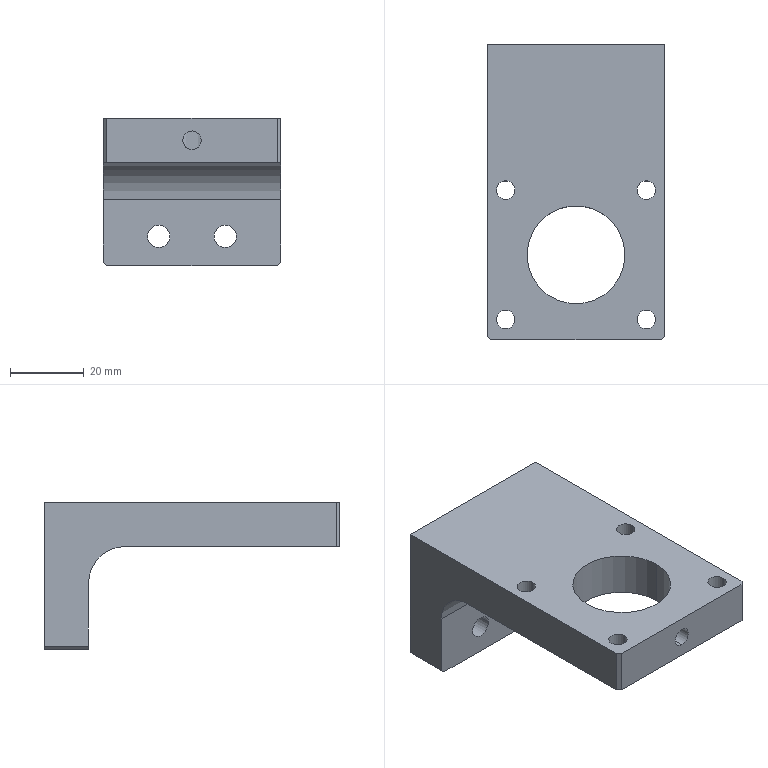Part | NX | features BREP 1 | 1 solid | 29 faces | box 48 x 80 x 40 mm | volume 54782 mm3 | cylinder 17 | plane 12 | commonest cylinder face diameters 5 x10 6 x4 26.5 x2 20 x1
STEP:
#1=CARTESIAN_POINT('',(0.,-30.25,2.5));
#2=VERTEX_POINT('',#1);
#3=CARTESIAN_POINT('',(0.,-30.25,-2.5));
#4=VERTEX_POINT('',#3);
#5=CARTESIAN_POINT('',(0.,-30.25,-2.5));
#6=CARTESIAN_POINT('',(-0.1554,-30.25,-2.5));
#7=CARTESIAN_POINT('',(-0.4644,-30.245,-2.477));
#8=CARTESIAN_POINT('',(-1.001,-30.214,-2.304));
#9=CARTESIAN_POINT('',(-1.293,-30.188,-2.154));
#10=CARTESIAN_POINT('',(-1.79,-30.132,-1.79));
#11=CARTESIAN_POINT('',(-2.16,-30.074,-1.284));
#12=CARTESIAN_POINT('',(-2.305,-30.048,-0.9992));
#13=CARTESIAN_POINT('',(-2.478,-30.017,-0.4608));
#14=CARTESIAN_POINT('',(-2.511,-30.01,0.001274));
#15=CARTESIAN_POINT('',(-2.478,-30.017,0.4638));
#16=CARTESIAN_POINT('',(-2.304,-30.048,1.002));
#17=CARTESIAN_POINT('',(-2.159,-30.074,1.286));
#18=CARTESIAN_POINT('',(-1.788,-30.132,1.793));
#19=CARTESIAN_POINT('',(-1.291,-30.188,2.155));
#20=CARTESIAN_POINT('',(-0.9972,-30.215,2.306));
#21=CARTESIAN_POINT('',(-0.4632,-30.245,2.477));
#22=CARTESIAN_POINT('',(-0.155,-30.25,2.5));
#23=CARTESIAN_POINT('',(0.,-30.25,2.5));
#24=B_SPLINE_CURVE_WITH_KNOTS('',3,(#5,#6,#7,#8,#9,#10,#11,#12,#13,#14,#15,#16,#17,#18,#19,#20,#21,#22,#23),.UNSPECIFIED.,.F.,.F.,(4,1,1,1,1,1,1,1,1,1,1,1,1,1,1,1,4),(0.,0.0625,0.125,0.1875,0.25,0.3125,0.375,0.4375,0.5,0.5625,0.625,0.6875,0.75,0.8125,0.875,0.9375,1.),.UNSPECIFIED.);
#25=EDGE_CURVE('',#2,#4,#24,.F.);
#26=ORIENTED_EDGE('',*,*,#25,.F.);
#27=CARTESIAN_POINT('',(0.,-40.,2.5));
#28=VERTEX_POINT('',#27);
#29=CARTESIAN_POINT('',(0.,-40.,2.5));
#30=DIRECTION('',(0.,-1.,0.));
#31=VECTOR('',#30,1000.);
#32=LINE('',#29,#31);
#33=EDGE_CURVE('',#2,#28,#32,.T.);
#34=ORIENTED_EDGE('',*,*,#33,.T.);
#35=CARTESIAN_POINT('',(0.,-40.,-2.5));
#36=VERTEX_POINT('',#35);
#37=CARTESIAN_POINT('',(0.,-40.,0.));
#38=DIRECTION('',(0.,-1.,0.));
#39=DIRECTION('',(0.,0.,-1.));
#40=AXIS2_PLACEMENT_3D('',#37,#38,#39);
#41=CIRCLE('',#40,2.5);
#42=EDGE_CURVE('',#28,#36,#41,.T.);
#43=ORIENTED_EDGE('',*,*,#42,.T.);
#44=CARTESIAN_POINT('',(0.,-40.,-2.5));
#45=DIRECTION('',(0.,-1.,0.));
#46=VECTOR('',#45,1000.);
#47=LINE('',#44,#46);
#48=EDGE_CURVE('',#4,#36,#47,.T.);
#49=ORIENTED_EDGE('',*,*,#48,.F.);
#50=EDGE_LOOP('',(#26,#34,#43,#49));
#51=FACE_BOUND('',#50,.T.);
#52=CARTESIAN_POINT('',(0.,-40.,0.));
#53=DIRECTION('',(0.,-1.,0.));
#54=DIRECTION('',(0.,0.,-1.));
#55=AXIS2_PLACEMENT_3D('',#52,#53,#54);
#56=CYLINDRICAL_SURFACE('',#55,2.5);
#57=ADVANCED_FACE('',(#51),#56,.F.);
#58=CARTESIAN_POINT('',(21.5,-34.5,6.));
#59=VERTEX_POINT('',#58);
#60=CARTESIAN_POINT('',(16.5,-34.5,6.));
#61=VERTEX_POINT('',#60);
#62=CARTESIAN_POINT('',(19.,-34.5,6.));
#63=DIRECTION('',(0.,0.,-1.));
#64=DIRECTION('',(1.,0.,0.));
#65=AXIS2_PLACEMENT_3D('',#62,#63,#64);
#66=CIRCLE('',#65,2.5);
#67=EDGE_CURVE('',#59,#61,#66,.T.);
#68=ORIENTED_EDGE('',*,*,#67,.F.);
#69=CARTESIAN_POINT('',(21.5,-34.5,-6.));
#70=VERTEX_POINT('',#69);
#71=CARTESIAN_POINT('',(21.5,-34.5,6.));
#72=DIRECTION('',(0.,0.,-1.));
#73=VECTOR('',#72,1000.);
#74=LINE('',#71,#73);
#75=EDGE_CURVE('',#59,#70,#74,.T.);
#76=ORIENTED_EDGE('',*,*,#75,.T.);
#77=CARTESIAN_POINT('',(16.5,-34.5,-6.));
#78=VERTEX_POINT('',#77);
#79=CARTESIAN_POINT('',(19.,-34.5,-6.));
#80=DIRECTION('',(0.,0.,-1.));
#81=DIRECTION('',(1.,0.,0.));
#82=AXIS2_PLACEMENT_3D('',#79,#80,#81);
#83=CIRCLE('',#82,2.5);
#84=EDGE_CURVE('',#70,#78,#83,.T.);
#85=ORIENTED_EDGE('',*,*,#84,.T.);
#86=CARTESIAN_POINT('',(16.5,-34.5,6.));
#87=DIRECTION('',(0.,0.,-1.));
#88=VECTOR('',#87,1000.);
#89=LINE('',#86,#88);
#90=EDGE_CURVE('',#61,#78,#89,.T.);
#91=ORIENTED_EDGE('',*,*,#90,.F.);
#92=EDGE_LOOP('',(#68,#76,#85,#91));
#93=FACE_BOUND('',#92,.T.);
#94=CARTESIAN_POINT('',(19.,-34.5,6.));
#95=DIRECTION('',(0.,0.,-1.));
#96=DIRECTION('',(-1.,0.,0.));
#97=AXIS2_PLACEMENT_3D('',#94,#95,#96);
#98=CYLINDRICAL_SURFACE('',#97,2.5);
#99=ADVANCED_FACE('',(#93),#98,.F.);
#100=CARTESIAN_POINT('',(21.5,0.5,6.));
#101=VERTEX_POINT('',#100);
#102=CARTESIAN_POINT('',(16.5,0.5,6.));
#103=VERTEX_POINT('',#102);
#104=CARTESIAN_POINT('',(19.,0.5,6.));
#105=DIRECTION('',(0.,0.,-1.));
#106=DIRECTION('',(1.,0.,0.));
#107=AXIS2_PLACEMENT_3D('',#104,#105,#106);
#108=CIRCLE('',#107,2.5);
#109=EDGE_CURVE('',#101,#103,#108,.T.);
#110=ORIENTED_EDGE('',*,*,#109,.F.);
#111=CARTESIAN_POINT('',(21.5,0.5,-6.));
#112=VERTEX_POINT('',#111);
#113=CARTESIAN_POINT('',(21.5,0.5,6.));
#114=DIRECTION('',(0.,0.,-1.));
#115=VECTOR('',#114,1000.);
#116=LINE('',#113,#115);
#117=EDGE_CURVE('',#101,#112,#116,.T.);
#118=ORIENTED_EDGE('',*,*,#117,.T.);
#119=CARTESIAN_POINT('',(16.5,0.5,-6.));
#120=VERTEX_POINT('',#119);
#121=CARTESIAN_POINT('',(19.,0.5,-6.));
#122=DIRECTION('',(0.,0.,-1.));
#123=DIRECTION('',(1.,0.,0.));
#124=AXIS2_PLACEMENT_3D('',#121,#122,#123);
#125=CIRCLE('',#124,2.5);
#126=EDGE_CURVE('',#112,#120,#125,.T.);
#127=ORIENTED_EDGE('',*,*,#126,.T.);
#128=CARTESIAN_POINT('',(16.5,0.5,6.));
#129=DIRECTION('',(0.,0.,-1.));
#130=VECTOR('',#129,1000.);
#131=LINE('',#128,#130);
#132=EDGE_CURVE('',#103,#120,#131,.T.);
#133=ORIENTED_EDGE('',*,*,#132,.F.);
#134=EDGE_LOOP('',(#110,#118,#127,#133));
#135=FACE_BOUND('',#134,.T.);
#136=CARTESIAN_POINT('',(19.,0.5,6.));
#137=DIRECTION('',(0.,0.,-1.));
#138=DIRECTION('',(-1.,0.,0.));
#139=AXIS2_PLACEMENT_3D('',#136,#137,#138);
#140=CYLINDRICAL_SURFACE('',#139,2.5);
#141=ADVANCED_FACE('',(#135),#140,.F.);
#142=CARTESIAN_POINT('',(-16.5,0.5,6.));
#143=VERTEX_POINT('',#142);
#144=CARTESIAN_POINT('',(-21.5,0.5,6.));
#145=VERTEX_POINT('',#144);
#146=CARTESIAN_POINT('',(-19.,0.5,6.));
#147=DIRECTION('',(0.,0.,-1.));
#148=DIRECTION('',(-1.,0.,0.));
#149=AXIS2_PLACEMENT_3D('',#146,#147,#148);
#150=CIRCLE('',#149,2.5);
#151=EDGE_CURVE('',#143,#145,#150,.T.);
#152=ORIENTED_EDGE('',*,*,#151,.F.);
#153=CARTESIAN_POINT('',(-16.5,0.5,-6.));
#154=VERTEX_POINT('',#153);
#155=CARTESIAN_POINT('',(-16.5,0.5,6.));
#156=DIRECTION('',(0.,0.,-1.));
#157=VECTOR('',#156,1000.);
#158=LINE('',#155,#157);
#159=EDGE_CURVE('',#143,#154,#158,.T.);
#160=ORIENTED_EDGE('',*,*,#159,.T.);
#161=CARTESIAN_POINT('',(-21.5,0.5,-6.));
#162=VERTEX_POINT('',#161);
#163=CARTESIAN_POINT('',(-19.,0.5,-6.));
#164=DIRECTION('',(0.,0.,-1.));
#165=DIRECTION('',(-1.,0.,0.));
#166=AXIS2_PLACEMENT_3D('',#163,#164,#165);
#167=CIRCLE('',#166,2.5);
#168=EDGE_CURVE('',#154,#162,#167,.T.);
#169=ORIENTED_EDGE('',*,*,#168,.T.);
#170=CARTESIAN_POINT('',(-21.5,0.5,6.));
#171=DIRECTION('',(0.,0.,-1.));
#172=VECTOR('',#171,1000.);
#173=LINE('',#170,#172);
#174=EDGE_CURVE('',#145,#162,#173,.T.);
#175=ORIENTED_EDGE('',*,*,#174,.F.);
#176=EDGE_LOOP('',(#152,#160,#169,#175));
#177=FACE_BOUND('',#176,.T.);
#178=CARTESIAN_POINT('',(-19.,0.5,6.));
#179=DIRECTION('',(0.,0.,-1.));
#180=DIRECTION('',(-1.,0.,0.));
#181=AXIS2_PLACEMENT_3D('',#178,#179,#180);
#182=CYLINDRICAL_SURFACE('',#181,2.5);
#183=ADVANCED_FACE('',(#177),#182,.F.);
#184=CARTESIAN_POINT('',(-16.5,-34.5,6.));
#185=VERTEX_POINT('',#184);
#186=CARTESIAN_POINT('',(-21.5,-34.5,6.));
#187=VERTEX_POINT('',#186);
#188=CARTESIAN_POINT('',(-19.,-34.5,6.));
#189=DIRECTION('',(0.,0.,-1.));
#190=DIRECTION('',(-1.,0.,0.));
#191=AXIS2_PLACEMENT_3D('',#188,#189,#190);
#192=CIRCLE('',#191,2.5);
#193=EDGE_CURVE('',#185,#187,#192,.T.);
#194=ORIENTED_EDGE('',*,*,#193,.F.);
#195=CARTESIAN_POINT('',(-16.5,-34.5,-6.));
#196=VERTEX_POINT('',#195);
#197=CARTESIAN_POINT('',(-16.5,-34.5,6.));
#198=DIRECTION('',(0.,0.,-1.));
#199=VECTOR('',#198,1000.);
#200=LINE('',#197,#199);
#201=EDGE_CURVE('',#185,#196,#200,.T.);
#202=ORIENTED_EDGE('',*,*,#201,.T.);
#203=CARTESIAN_POINT('',(-21.5,-34.5,-6.));
#204=VERTEX_POINT('',#203);
#205=CARTESIAN_POINT('',(-19.,-34.5,-6.));
#206=DIRECTION('',(0.,0.,-1.));
#207=DIRECTION('',(-1.,0.,0.));
#208=AXIS2_PLACEMENT_3D('',#205,#206,#207);
#209=CIRCLE('',#208,2.5);
#210=EDGE_CURVE('',#196,#204,#209,.T.);
#211=ORIENTED_EDGE('',*,*,#210,.T.);
#212=CARTESIAN_POINT('',(-21.5,-34.5,6.));
#213=DIRECTION('',(0.,0.,-1.));
#214=VECTOR('',#213,1000.);
#215=LINE('',#212,#214);
#216=EDGE_CURVE('',#187,#204,#215,.T.);
#217=ORIENTED_EDGE('',*,*,#216,.F.);
#218=EDGE_LOOP('',(#194,#202,#211,#217));
#219=FACE_BOUND('',#218,.T.);
#220=CARTESIAN_POINT('',(-19.,-34.5,6.));
#221=DIRECTION('',(0.,0.,-1.));
#222=DIRECTION('',(-1.,0.,0.));
#223=AXIS2_PLACEMENT_3D('',#220,#221,#222);
#224=CYLINDRICAL_SURFACE('',#223,2.5);
#225=ADVANCED_FACE('',(#219),#224,.F.);
#226=CARTESIAN_POINT('',(6.,40.,-26.));
#227=VERTEX_POINT('',#226);
#228=CARTESIAN_POINT('',(12.,40.,-26.));
#229=VERTEX_POINT('',#228);
#230=CARTESIAN_POINT('',(9.,40.,-26.));
#231=DIRECTION('',(0.,-1.,0.));
#232=DIRECTION('',(0.,0.,-1.));
#233=AXIS2_PLACEMENT_3D('',#230,#231,#232);
#234=CIRCLE('',#233,3.);
#235=EDGE_CURVE('',#227,#229,#234,.T.);
#236=ORIENTED_EDGE('',*,*,#235,.F.);
#237=CARTESIAN_POINT('',(6.,28.,-26.));
#238=VERTEX_POINT('',#237);
#239=CARTESIAN_POINT('',(6.,58.,-26.));
#240=DIRECTION('',(0.,-1.,0.));
#241=VECTOR('',#240,1000.);
#242=LINE('',#239,#241);
#243=EDGE_CURVE('',#238,#227,#242,.F.);
#244=ORIENTED_EDGE('',*,*,#243,.F.);
#245=CARTESIAN_POINT('',(12.,28.,-26.));
#246=VERTEX_POINT('',#245);
#247=CARTESIAN_POINT('',(9.,28.,-26.));
#248=DIRECTION('',(0.,-1.,0.));
#249=DIRECTION('',(1.,0.,0.));
#250=AXIS2_PLACEMENT_3D('',#247,#248,#249);
#251=CIRCLE('',#250,3.);
#252=EDGE_CURVE('',#238,#246,#251,.T.);
#253=ORIENTED_EDGE('',*,*,#252,.T.);
#254=CARTESIAN_POINT('',(12.,58.,-26.));
#255=DIRECTION('',(0.,-1.,0.));
#256=VECTOR('',#255,1000.);
#257=LINE('',#254,#256);
#258=EDGE_CURVE('',#246,#229,#257,.F.);
#259=ORIENTED_EDGE('',*,*,#258,.T.);
#260=EDGE_LOOP('',(#236,#244,#253,#259));
#261=FACE_BOUND('',#260,.T.);
#262=CARTESIAN_POINT('',(9.,58.,-26.));
#263=DIRECTION('',(0.,-1.,0.));
#264=DIRECTION('',(1.,0.,0.));
#265=AXIS2_PLACEMENT_3D('',#262,#263,#264);
#266=CYLINDRICAL_SURFACE('',#265,3.);
#267=ADVANCED_FACE('',(#261),#266,.F.);
#268=CARTESIAN_POINT('',(-12.,40.,-26.));
#269=VERTEX_POINT('',#268);
#270=CARTESIAN_POINT('',(-6.,40.,-26.));
#271=VERTEX_POINT('',#270);
#272=CARTESIAN_POINT('',(-9.,40.,-26.));
#273=DIRECTION('',(0.,-1.,0.));
#274=DIRECTION('',(0.,0.,-1.));
#275=AXIS2_PLACEMENT_3D('',#272,#273,#274);
#276=CIRCLE('',#275,3.);
#277=EDGE_CURVE('',#269,#271,#276,.T.);
#278=ORIENTED_EDGE('',*,*,#277,.F.);
#279=CARTESIAN_POINT('',(-12.,28.,-26.));
#280=VERTEX_POINT('',#279);
#281=CARTESIAN_POINT('',(-12.,58.,-26.));
#282=DIRECTION('',(0.,-1.,0.));
#283=VECTOR('',#282,1000.);
#284=LINE('',#281,#283);
#285=EDGE_CURVE('',#280,#269,#284,.F.);
#286=ORIENTED_EDGE('',*,*,#285,.F.);
#287=CARTESIAN_POINT('',(-6.,28.,-26.));
#288=VERTEX_POINT('',#287);
#289=CARTESIAN_POINT('',(-9.,28.,-26.));
#290=DIRECTION('',(0.,-1.,0.));
#291=DIRECTION('',(1.,0.,0.));
#292=AXIS2_PLACEMENT_3D('',#289,#290,#291);
#293=CIRCLE('',#292,3.);
#294=EDGE_CURVE('',#280,#288,#293,.T.);
#295=ORIENTED_EDGE('',*,*,#294,.T.);
#296=CARTESIAN_POINT('',(-6.,58.,-26.));
#297=DIRECTION('',(0.,-1.,0.));
#298=VECTOR('',#297,1000.);
#299=LINE('',#296,#298);
#300=EDGE_CURVE('',#288,#271,#299,.F.);
#301=ORIENTED_EDGE('',*,*,#300,.T.);
#302=EDGE_LOOP('',(#278,#286,#295,#301));
#303=FACE_BOUND('',#302,.T.);
#304=CARTESIAN_POINT('',(-9.,58.,-26.));
#305=DIRECTION('',(0.,-1.,0.));
#306=DIRECTION('',(1.,0.,0.));
#307=AXIS2_PLACEMENT_3D('',#304,#305,#306);
#308=CYLINDRICAL_SURFACE('',#307,3.);
#309=ADVANCED_FACE('',(#303),#308,.F.);
#310=CARTESIAN_POINT('',(-13.25,-17.,-6.));
#311=VERTEX_POINT('',#310);
#312=CARTESIAN_POINT('',(13.25,-17.,-6.));
#313=VERTEX_POINT('',#312);
#314=CARTESIAN_POINT('',(0.,-17.,-6.));
#315=DIRECTION('',(0.,0.,1.));
#316=DIRECTION('',(1.,0.,0.));
#317=AXIS2_PLACEMENT_3D('',#314,#315,#316);
#318=CIRCLE('',#317,13.25);
#319=EDGE_CURVE('',#311,#313,#318,.T.);
#320=ORIENTED_EDGE('',*,*,#319,.F.);
#321=CARTESIAN_POINT('',(-13.25,-17.,6.));
#322=VERTEX_POINT('',#321);
#323=CARTESIAN_POINT('',(-13.25,-17.,-6.));
#324=DIRECTION('',(0.,0.,1.));
#325=VECTOR('',#324,1000.);
#326=LINE('',#323,#325);
#327=EDGE_CURVE('',#322,#311,#326,.F.);
#328=ORIENTED_EDGE('',*,*,#327,.F.);
#329=CARTESIAN_POINT('',(13.25,-17.,6.));
#330=VERTEX_POINT('',#329);
#331=CARTESIAN_POINT('',(0.,-17.,6.));
#332=DIRECTION('',(0.,0.,1.));
#333=DIRECTION('',(1.,0.,0.));
#334=AXIS2_PLACEMENT_3D('',#331,#332,#333);
#335=CIRCLE('',#334,13.25);
#336=EDGE_CURVE('',#322,#330,#335,.T.);
#337=ORIENTED_EDGE('',*,*,#336,.T.);
#338=CARTESIAN_POINT('',(13.25,-17.,-6.));
#339=DIRECTION('',(0.,0.,1.));
#340=VECTOR('',#339,1000.);
#341=LINE('',#338,#340);
#342=EDGE_CURVE('',#330,#313,#341,.F.);
#343=ORIENTED_EDGE('',*,*,#342,.T.);
#344=EDGE_LOOP('',(#320,#328,#337,#343));
#345=FACE_BOUND('',#344,.T.);
#346=CARTESIAN_POINT('',(0.,-30.25,-2.5));
#347=CARTESIAN_POINT('',(0.6639,-30.25,-2.5));
#348=CARTESIAN_POINT('',(1.954,-30.132,-1.958));
#349=CARTESIAN_POINT('',(2.773,-29.952,-0.001957));
#350=CARTESIAN_POINT('',(1.954,-30.132,1.96));
#351=CARTESIAN_POINT('',(0.6633,-30.25,2.5));
#352=CARTESIAN_POINT('',(0.,-30.25,2.5));
#353=B_SPLINE_CURVE_WITH_KNOTS('',3,(#346,#347,#348,#349,#350,#351,#352),.UNSPECIFIED.,.F.,.F.,(4,1,1,1,4),(0.,0.25,0.5,0.75,1.),.UNSPECIFIED.);
#354=EDGE_CURVE('',#4,#2,#353,.T.);
#355=ORIENTED_EDGE('',*,*,#354,.T.);
#356=ORIENTED_EDGE('',*,*,#25,.T.);
#357=EDGE_LOOP('',(#355,#356));
#358=FACE_BOUND('',#357,.T.);
#359=CARTESIAN_POINT('',(0.,-17.,-6.));
#360=DIRECTION('',(0.,0.,1.));
#361=DIRECTION('',(1.,0.,0.));
#362=AXIS2_PLACEMENT_3D('',#359,#360,#361);
#363=CYLINDRICAL_SURFACE('',#362,13.25);
#364=ADVANCED_FACE('',(#345,#358),#363,.F.);
#365=CARTESIAN_POINT('',(-24.,18.,-6.));
#366=VERTEX_POINT('',#365);
#367=CARTESIAN_POINT('',(-24.,-39.,-6.));
#368=VERTEX_POINT('',#367);
#369=CARTESIAN_POINT('',(-24.,-40.,-6.));
#370=DIRECTION('',(0.,-1.,0.));
#371=VECTOR('',#370,1000.);
#372=LINE('',#369,#371);
#373=EDGE_CURVE('',#366,#368,#372,.T.);
#374=ORIENTED_EDGE('',*,*,#373,.F.);
#375=CARTESIAN_POINT('',(24.,18.,-6.));
#376=VERTEX_POINT('',#375);
#377=CARTESIAN_POINT('',(24.,18.,-6.));
#378=DIRECTION('',(1.,0.,0.));
#379=VECTOR('',#378,1000.);
#380=LINE('',#377,#379);
#381=EDGE_CURVE('',#366,#376,#380,.T.);
#382=ORIENTED_EDGE('',*,*,#381,.T.);
#383=CARTESIAN_POINT('',(24.,-39.,-6.));
#384=VERTEX_POINT('',#383);
#385=CARTESIAN_POINT('',(24.,-40.,-6.));
#386=DIRECTION('',(0.,1.,0.));
#387=VECTOR('',#386,1000.);
#388=LINE('',#385,#387);
#389=EDGE_CURVE('',#384,#376,#388,.T.);
#390=ORIENTED_EDGE('',*,*,#389,.F.);
#391=CARTESIAN_POINT('',(23.,-40.,-6.));
#392=VERTEX_POINT('',#391);
#393=CARTESIAN_POINT('',(24.,-39.,-6.));
#394=DIRECTION('',(-0.7071,-0.7071,0.));
#395=VECTOR('',#394,1000.);
#396=LINE('',#393,#395);
#397=EDGE_CURVE('',#384,#392,#396,.T.);
#398=ORIENTED_EDGE('',*,*,#397,.T.);
#399=CARTESIAN_POINT('',(-23.,-40.,-6.));
#400=VERTEX_POINT('',#399);
#401=CARTESIAN_POINT('',(24.,-40.,-6.));
#402=DIRECTION('',(1.,0.,0.));
#403=VECTOR('',#402,1000.);
#404=LINE('',#401,#403);
#405=EDGE_CURVE('',#400,#392,#404,.T.);
#406=ORIENTED_EDGE('',*,*,#405,.F.);
#407=CARTESIAN_POINT('',(-23.,-40.,-6.));
#408=DIRECTION('',(-0.7071,0.7071,0.));
#409=VECTOR('',#408,1000.);
#410=LINE('',#407,#409);
#411=EDGE_CURVE('',#400,#368,#410,.T.);
#412=ORIENTED_EDGE('',*,*,#411,.T.);
#413=EDGE_LOOP('',(#374,#382,#390,#398,#406,#412));
#414=FACE_BOUND('',#413,.T.);
#415=CARTESIAN_POINT('',(19.,-34.5,-6.));
#416=DIRECTION('',(0.,0.,-1.));
#417=DIRECTION('',(1.,0.,0.));
#418=AXIS2_PLACEMENT_3D('',#415,#416,#417);
#419=CIRCLE('',#418,2.5);
#420=EDGE_CURVE('',#78,#70,#419,.T.);
#421=ORIENTED_EDGE('',*,*,#420,.F.);
#422=ORIENTED_EDGE('',*,*,#84,.F.);
#423=EDGE_LOOP('',(#421,#422));
#424=FACE_BOUND('',#423,.T.);
#425=CARTESIAN_POINT('',(19.,0.5,-6.));
#426=DIRECTION('',(0.,0.,-1.));
#427=DIRECTION('',(1.,0.,0.));
#428=AXIS2_PLACEMENT_3D('',#425,#426,#427);
#429=CIRCLE('',#428,2.5);
#430=EDGE_CURVE('',#120,#112,#429,.T.);
#431=ORIENTED_EDGE('',*,*,#430,.F.);
#432=ORIENTED_EDGE('',*,*,#126,.F.);
#433=EDGE_LOOP('',(#431,#432));
#434=FACE_BOUND('',#433,.T.);
#435=CARTESIAN_POINT('',(-19.,0.5,-6.));
#436=DIRECTION('',(0.,0.,-1.));
#437=DIRECTION('',(-1.,0.,0.));
#438=AXIS2_PLACEMENT_3D('',#435,#436,#437);
#439=CIRCLE('',#438,2.5);
#440=EDGE_CURVE('',#162,#154,#439,.T.);
#441=ORIENTED_EDGE('',*,*,#440,.F.);
#442=ORIENTED_EDGE('',*,*,#168,.F.);
#443=EDGE_LOOP('',(#441,#442));
#444=FACE_BOUND('',#443,.T.);
#445=CARTESIAN_POINT('',(-19.,-34.5,-6.));
#446=DIRECTION('',(0.,0.,-1.));
#447=DIRECTION('',(-1.,0.,0.));
#448=AXIS2_PLACEMENT_3D('',#445,#446,#447);
#449=CIRCLE('',#448,2.5);
#450=EDGE_CURVE('',#204,#196,#449,.T.);
#451=ORIENTED_EDGE('',*,*,#450,.F.);
#452=ORIENTED_EDGE('',*,*,#210,.F.);
#453=EDGE_LOOP('',(#451,#452));
#454=FACE_BOUND('',#453,.T.);
#455=CARTESIAN_POINT('',(0.,-17.,-6.));
#456=DIRECTION('',(0.,0.,1.));
#457=DIRECTION('',(1.,0.,0.));
#458=AXIS2_PLACEMENT_3D('',#455,#456,#457);
#459=CIRCLE('',#458,13.25);
#460=EDGE_CURVE('',#313,#311,#459,.T.);
#461=ORIENTED_EDGE('',*,*,#460,.T.);
#462=ORIENTED_EDGE('',*,*,#319,.T.);
#463=EDGE_LOOP('',(#461,#462));
#464=FACE_BOUND('',#463,.T.);
#465=CARTESIAN_POINT('',(0.,0.,-6.));
#466=DIRECTION('',(0.,0.,1.));
#467=DIRECTION('',(1.,0.,0.));
#468=AXIS2_PLACEMENT_3D('',#465,#466,#467);
#469=PLANE('',#468);
#470=ADVANCED_FACE('',(#414,#424,#434,#444,#454,#464),#469,.F.);
#471=CARTESIAN_POINT('',(-24.,40.,6.));
#472=VERTEX_POINT('',#471);
#473=CARTESIAN_POINT('',(-24.,40.,-33.));
#474=VERTEX_POINT('',#473);
#475=CARTESIAN_POINT('',(-24.,40.,6.));
#476=DIRECTION('',(0.,0.,-1.));
#477=VECTOR('',#476,1000.);
#478=LINE('',#475,#477);
#479=EDGE_CURVE('',#472,#474,#478,.T.);
#480=ORIENTED_EDGE('',*,*,#479,.T.);
#481=CARTESIAN_POINT('',(-24.,28.,-33.));
#482=VERTEX_POINT('',#481);
#483=CARTESIAN_POINT('',(-24.,-40.,-33.));
#484=DIRECTION('',(0.,-1.,0.));
#485=VECTOR('',#484,1000.);
#486=LINE('',#483,#485);
#487=EDGE_CURVE('',#474,#482,#486,.T.);
#488=ORIENTED_EDGE('',*,*,#487,.T.);
#489=CARTESIAN_POINT('',(-24.,28.,-16.));
#490=VERTEX_POINT('',#489);
#491=CARTESIAN_POINT('',(-24.,28.,-34.));
#492=DIRECTION('',(0.,0.,1.));
#493=VECTOR('',#492,1000.);
#494=LINE('',#491,#493);
#495=EDGE_CURVE('',#482,#490,#494,.T.);
#496=ORIENTED_EDGE('',*,*,#495,.T.);
#497=CARTESIAN_POINT('',(-24.,18.,-16.));
#498=DIRECTION('',(1.,0.,0.));
#499=DIRECTION('',(0.,0.,-1.));
#500=AXIS2_PLACEMENT_3D('',#497,#498,#499);
#501=CIRCLE('',#500,10.);
#502=EDGE_CURVE('',#490,#366,#501,.T.);
#503=ORIENTED_EDGE('',*,*,#502,.T.);
#504=ORIENTED_EDGE('',*,*,#373,.T.);
#505=CARTESIAN_POINT('',(-24.,-39.,6.));
#506=VERTEX_POINT('',#505);
#507=CARTESIAN_POINT('',(-24.,-39.,6.));
#508=DIRECTION('',(0.,0.,1.));
#509=VECTOR('',#508,1000.);
#510=LINE('',#507,#509);
#511=EDGE_CURVE('',#368,#506,#510,.T.);
#512=ORIENTED_EDGE('',*,*,#511,.T.);
#513=CARTESIAN_POINT('',(-24.,-40.,6.));
#514=DIRECTION('',(0.,-1.,0.));
#515=VECTOR('',#514,1000.);
#516=LINE('',#513,#515);
#517=EDGE_CURVE('',#472,#506,#516,.T.);
#518=ORIENTED_EDGE('',*,*,#517,.F.);
#519=EDGE_LOOP('',(#480,#488,#496,#503,#504,#512,#518));
#520=FACE_BOUND('',#519,.T.);
#521=CARTESIAN_POINT('',(-24.,-40.,6.));
#522=DIRECTION('',(1.,0.,0.));
#523=DIRECTION('',(0.,1.,0.));
#524=AXIS2_PLACEMENT_3D('',#521,#522,#523);
#525=PLANE('',#524);
#526=ADVANCED_FACE('',(#520),#525,.F.);
#527=ORIENTED_EDGE('',*,*,#405,.T.);
#528=CARTESIAN_POINT('',(23.,-40.,6.));
#529=VERTEX_POINT('',#528);
#530=CARTESIAN_POINT('',(23.,-40.,6.));
#531=DIRECTION('',(0.,0.,1.));
#532=VECTOR('',#531,1000.);
#533=LINE('',#530,#532);
#534=EDGE_CURVE('',#392,#529,#533,.T.);
#535=ORIENTED_EDGE('',*,*,#534,.T.);
#536=CARTESIAN_POINT('',(-23.,-40.,6.));
#537=VERTEX_POINT('',#536);
#538=CARTESIAN_POINT('',(24.,-40.,6.));
#539=DIRECTION('',(1.,0.,0.));
#540=VECTOR('',#539,1000.);
#541=LINE('',#538,#540);
#542=EDGE_CURVE('',#537,#529,#541,.T.);
#543=ORIENTED_EDGE('',*,*,#542,.F.);
#544=CARTESIAN_POINT('',(-23.,-40.,6.));
#545=DIRECTION('',(0.,0.,-1.));
#546=VECTOR('',#545,1000.);
#547=LINE('',#544,#546);
#548=EDGE_CURVE('',#537,#400,#547,.T.);
#549=ORIENTED_EDGE('',*,*,#548,.T.);
#550=EDGE_LOOP('',(#527,#535,#543,#549));
#551=FACE_BOUND('',#550,.T.);
#552=CARTESIAN_POINT('',(0.,-40.,0.));
#553=DIRECTION('',(0.,-1.,0.));
#554=DIRECTION('',(0.,0.,-1.));
#555=AXIS2_PLACEMENT_3D('',#552,#553,#554);
#556=CIRCLE('',#555,2.5);
#557=EDGE_CURVE('',#36,#28,#556,.T.);
#558=ORIENTED_EDGE('',*,*,#557,.F.);
#559=ORIENTED_EDGE('',*,*,#42,.F.);
#560=EDGE_LOOP('',(#558,#559));
#561=FACE_BOUND('',#560,.T.);
#562=CARTESIAN_POINT('',(24.,-40.,6.));
#563=DIRECTION('',(0.,1.,0.));
#564=DIRECTION('',(1.,0.,0.));
#565=AXIS2_PLACEMENT_3D('',#562,#563,#564);
#566=PLANE('',#565);
#567=ADVANCED_FACE('',(#551,#561),#566,.F.);
#568=CARTESIAN_POINT('',(24.,28.,-33.));
#569=VERTEX_POINT('',#568);
#570=CARTESIAN_POINT('',(24.,28.,-16.));
#571=VERTEX_POINT('',#570);
#572=CARTESIAN_POINT('',(24.,28.,-34.));
#573=DIRECTION('',(0.,0.,1.));
#574=VECTOR('',#573,1000.);
#575=LINE('',#572,#574);
#576=EDGE_CURVE('',#569,#571,#575,.T.);
#577=ORIENTED_EDGE('',*,*,#576,.F.);
#578=CARTESIAN_POINT('',(24.,40.,-33.));
#579=VERTEX_POINT('',#578);
#580=CARTESIAN_POINT('',(24.,-40.,-33.));
#581=DIRECTION('',(0.,1.,0.));
#582=VECTOR('',#581,1000.);
#583=LINE('',#580,#582);
#584=EDGE_CURVE('',#569,#579,#583,.T.);
#585=ORIENTED_EDGE('',*,*,#584,.T.);
#586=CARTESIAN_POINT('',(24.,40.,6.));
#587=VERTEX_POINT('',#586);
#588=CARTESIAN_POINT('',(24.,40.,6.));
#589=DIRECTION('',(0.,0.,-1.));
#590=VECTOR('',#589,1000.);
#591=LINE('',#588,#590);
#592=EDGE_CURVE('',#587,#579,#591,.T.);
#593=ORIENTED_EDGE('',*,*,#592,.F.);
#594=CARTESIAN_POINT('',(24.,-39.,6.));
#595=VERTEX_POINT('',#594);
#596=CARTESIAN_POINT('',(24.,-40.,6.));
#597=DIRECTION('',(0.,1.,0.));
#598=VECTOR('',#597,1000.);
#599=LINE('',#596,#598);
#600=EDGE_CURVE('',#595,#587,#599,.T.);
#601=ORIENTED_EDGE('',*,*,#600,.F.);
#602=CARTESIAN_POINT('',(24.,-39.,6.));
#603=DIRECTION('',(0.,0.,-1.));
#604=VECTOR('',#603,1000.);
#605=LINE('',#602,#604);
#606=EDGE_CURVE('',#595,#384,#605,.T.);
#607=ORIENTED_EDGE('',*,*,#606,.T.);
#608=ORIENTED_EDGE('',*,*,#389,.T.);
#609=CARTESIAN_POINT('',(24.,18.,-16.));
#610=DIRECTION('',(-1.,0.,0.));
#611=DIRECTION('',(0.,0.,1.));
#612=AXIS2_PLACEMENT_3D('',#609,#610,#611);
#613=CIRCLE('',#612,10.);
#614=EDGE_CURVE('',#376,#571,#613,.T.);
#615=ORIENTED_EDGE('',*,*,#614,.T.);
#616=EDGE_LOOP('',(#577,#585,#593,#601,#607,#608,#615));
#617=FACE_BOUND('',#616,.T.);
#618=CARTESIAN_POINT('',(24.,-40.,6.));
#619=DIRECTION('',(-1.,0.,0.));
#620=DIRECTION('',(0.,0.,1.));
#621=AXIS2_PLACEMENT_3D('',#618,#619,#620);
#622=PLANE('',#621);
#623=ADVANCED_FACE('',(#617),#622,.F.);
#624=CARTESIAN_POINT('',(-23.,40.,-34.));
#625=VERTEX_POINT('',#624);
#626=CARTESIAN_POINT('',(23.,40.,-34.));
#627=VERTEX_POINT('',#626);
#628=CARTESIAN_POINT('',(24.,40.,-34.));
#629=DIRECTION('',(1.,0.,0.));
#630=VECTOR('',#629,1000.);
#631=LINE('',#628,#630);
#632=EDGE_CURVE('',#625,#627,#631,.T.);
#633=ORIENTED_EDGE('',*,*,#632,.F.);
#634=CARTESIAN_POINT('',(-23.,40.,-34.));
#635=DIRECTION('',(-0.7071,0.,0.7071));
#636=VECTOR('',#635,1000.);
#637=LINE('',#634,#636);
#638=EDGE_CURVE('',#625,#474,#637,.T.);
#639=ORIENTED_EDGE('',*,*,#638,.T.);
#640=ORIENTED_EDGE('',*,*,#479,.F.);
#641=CARTESIAN_POINT('',(24.,40.,6.));
#642=DIRECTION('',(-1.,0.,0.));
#643=VECTOR('',#642,1000.);
#644=LINE('',#641,#643);
#645=EDGE_CURVE('',#587,#472,#644,.T.);
#646=ORIENTED_EDGE('',*,*,#645,.F.);
#647=ORIENTED_EDGE('',*,*,#592,.T.);
#648=CARTESIAN_POINT('',(23.,40.,-34.));
#649=DIRECTION('',(-0.7071,0.,-0.7071));
#650=VECTOR('',#649,1000.);
#651=LINE('',#648,#650);
#652=EDGE_CURVE('',#579,#627,#651,.T.);
#653=ORIENTED_EDGE('',*,*,#652,.T.);
#654=EDGE_LOOP('',(#633,#639,#640,#646,#647,#653));
#655=FACE_BOUND('',#654,.T.);
#656=CARTESIAN_POINT('',(9.,40.,-26.));
#657=DIRECTION('',(0.,-1.,0.));
#658=DIRECTION('',(0.,0.,-1.));
#659=AXIS2_PLACEMENT_3D('',#656,#657,#658);
#660=CIRCLE('',#659,3.);
#661=EDGE_CURVE('',#229,#227,#660,.T.);
#662=ORIENTED_EDGE('',*,*,#661,.T.);
#663=ORIENTED_EDGE('',*,*,#235,.T.);
#664=EDGE_LOOP('',(#662,#663));
#665=FACE_BOUND('',#664,.T.);
#666=CARTESIAN_POINT('',(-9.,40.,-26.));
#667=DIRECTION('',(0.,-1.,0.));
#668=DIRECTION('',(0.,0.,-1.));
#669=AXIS2_PLACEMENT_3D('',#666,#667,#668);
#670=CIRCLE('',#669,3.);
#671=EDGE_CURVE('',#271,#269,#670,.T.);
#672=ORIENTED_EDGE('',*,*,#671,.T.);
#673=ORIENTED_EDGE('',*,*,#277,.T.);
#674=EDGE_LOOP('',(#672,#673));
#675=FACE_BOUND('',#674,.T.);
#676=CARTESIAN_POINT('',(24.,40.,6.));
#677=DIRECTION('',(0.,-1.,0.));
#678=DIRECTION('',(0.,0.,-1.));
#679=AXIS2_PLACEMENT_3D('',#676,#677,#678);
#680=PLANE('',#679);
#681=ADVANCED_FACE('',(#655,#665,#675),#680,.F.);
#682=ORIENTED_EDGE('',*,*,#542,.T.);
#683=CARTESIAN_POINT('',(31.5,-31.5,6.));
#684=DIRECTION('',(0.7071,0.7071,0.));
#685=VECTOR('',#684,1000.);
#686=LINE('',#683,#685);
#687=EDGE_CURVE('',#529,#595,#686,.T.);
#688=ORIENTED_EDGE('',*,*,#687,.T.);
#689=ORIENTED_EDGE('',*,*,#600,.T.);
#690=ORIENTED_EDGE('',*,*,#645,.T.);
#691=ORIENTED_EDGE('',*,*,#517,.T.);
#692=CARTESIAN_POINT('',(-31.5,-31.5,6.));
#693=DIRECTION('',(0.7071,-0.7071,0.));
#694=VECTOR('',#693,1000.);
#695=LINE('',#692,#694);
#696=EDGE_CURVE('',#506,#537,#695,.T.);
#697=ORIENTED_EDGE('',*,*,#696,.T.);
#698=EDGE_LOOP('',(#682,#688,#689,#690,#691,#697));
#699=FACE_BOUND('',#698,.T.);
#700=CARTESIAN_POINT('',(19.,-34.5,6.));
#701=DIRECTION('',(0.,0.,-1.));
#702=DIRECTION('',(1.,0.,0.));
#703=AXIS2_PLACEMENT_3D('',#700,#701,#702);
#704=CIRCLE('',#703,2.5);
#705=EDGE_CURVE('',#61,#59,#704,.T.);
#706=ORIENTED_EDGE('',*,*,#705,.T.);
#707=ORIENTED_EDGE('',*,*,#67,.T.);
#708=EDGE_LOOP('',(#706,#707));
#709=FACE_BOUND('',#708,.T.);
#710=CARTESIAN_POINT('',(19.,0.5,6.));
#711=DIRECTION('',(0.,0.,-1.));
#712=DIRECTION('',(1.,0.,0.));
#713=AXIS2_PLACEMENT_3D('',#710,#711,#712);
#714=CIRCLE('',#713,2.5);
#715=EDGE_CURVE('',#103,#101,#714,.T.);
#716=ORIENTED_EDGE('',*,*,#715,.T.);
#717=ORIENTED_EDGE('',*,*,#109,.T.);
#718=EDGE_LOOP('',(#716,#717));
#719=FACE_BOUND('',#718,.T.);
#720=CARTESIAN_POINT('',(-19.,0.5,6.));
#721=DIRECTION('',(0.,0.,-1.));
#722=DIRECTION('',(-1.,0.,0.));
#723=AXIS2_PLACEMENT_3D('',#720,#721,#722);
#724=CIRCLE('',#723,2.5);
#725=EDGE_CURVE('',#145,#143,#724,.T.);
#726=ORIENTED_EDGE('',*,*,#725,.T.);
#727=ORIENTED_EDGE('',*,*,#151,.T.);
#728=EDGE_LOOP('',(#726,#727));
#729=FACE_BOUND('',#728,.T.);
#730=CARTESIAN_POINT('',(-19.,-34.5,6.));
#731=DIRECTION('',(0.,0.,-1.));
#732=DIRECTION('',(-1.,0.,0.));
#733=AXIS2_PLACEMENT_3D('',#730,#731,#732);
#734=CIRCLE('',#733,2.5);
#735=EDGE_CURVE('',#187,#185,#734,.T.);
#736=ORIENTED_EDGE('',*,*,#735,.T.);
#737=ORIENTED_EDGE('',*,*,#193,.T.);
#738=EDGE_LOOP('',(#736,#737));
#739=FACE_BOUND('',#738,.T.);
#740=CARTESIAN_POINT('',(0.,-17.,6.));
#741=DIRECTION('',(0.,0.,1.));
#742=DIRECTION('',(1.,0.,0.));
#743=AXIS2_PLACEMENT_3D('',#740,#741,#742);
#744=CIRCLE('',#743,13.25);
#745=EDGE_CURVE('',#330,#322,#744,.T.);
#746=ORIENTED_EDGE('',*,*,#745,.F.);
#747=ORIENTED_EDGE('',*,*,#336,.F.);
#748=EDGE_LOOP('',(#746,#747));
#749=FACE_BOUND('',#748,.T.);
#750=CARTESIAN_POINT('',(0.,0.,6.));
#751=DIRECTION('',(0.,0.,1.));
#752=DIRECTION('',(1.,0.,0.));
#753=AXIS2_PLACEMENT_3D('',#750,#751,#752);
#754=PLANE('',#753);
#755=ADVANCED_FACE('',(#699,#709,#719,#729,#739,#749),#754,.T.);
#756=ORIENTED_EDGE('',*,*,#327,.T.);
#757=ORIENTED_EDGE('',*,*,#460,.F.);
#758=ORIENTED_EDGE('',*,*,#342,.F.);
#759=ORIENTED_EDGE('',*,*,#745,.T.);
#760=EDGE_LOOP('',(#756,#757,#758,#759));
#761=FACE_BOUND('',#760,.T.);
#762=CARTESIAN_POINT('',(0.,-17.,-6.));
#763=DIRECTION('',(0.,0.,1.));
#764=DIRECTION('',(1.,0.,0.));
#765=AXIS2_PLACEMENT_3D('',#762,#763,#764);
#766=CYLINDRICAL_SURFACE('',#765,13.25);
#767=ADVANCED_FACE('',(#761),#766,.F.);
#768=ORIENTED_EDGE('',*,*,#687,.F.);
#769=ORIENTED_EDGE('',*,*,#534,.F.);
#770=ORIENTED_EDGE('',*,*,#397,.F.);
#771=ORIENTED_EDGE('',*,*,#606,.F.);
#772=EDGE_LOOP('',(#768,#769,#770,#771));
#773=FACE_BOUND('',#772,.T.);
#774=CARTESIAN_POINT('',(24.,-39.,6.));
#775=DIRECTION('',(-0.7071,0.7071,0.));
#776=DIRECTION('',(0.,0.,1.));
#777=AXIS2_PLACEMENT_3D('',#774,#775,#776);
#778=PLANE('',#777);
#779=ADVANCED_FACE('',(#773),#778,.F.);
#780=ORIENTED_EDGE('',*,*,#696,.F.);
#781=ORIENTED_EDGE('',*,*,#511,.F.);
#782=ORIENTED_EDGE('',*,*,#411,.F.);
#783=ORIENTED_EDGE('',*,*,#548,.F.);
#784=EDGE_LOOP('',(#780,#781,#782,#783));
#785=FACE_BOUND('',#784,.T.);
#786=CARTESIAN_POINT('',(-23.,-40.,6.));
#787=DIRECTION('',(0.7071,0.7071,0.));
#788=DIRECTION('',(0.,0.,-1.));
#789=AXIS2_PLACEMENT_3D('',#786,#787,#788);
#790=PLANE('',#789);
#791=ADVANCED_FACE('',(#785),#790,.F.);
#792=ORIENTED_EDGE('',*,*,#495,.F.);
#793=CARTESIAN_POINT('',(-23.,28.,-34.));
#794=VERTEX_POINT('',#793);
#795=CARTESIAN_POINT('',(-23.,28.,-34.));
#796=DIRECTION('',(0.7071,0.,-0.7071));
#797=VECTOR('',#796,1000.);
#798=LINE('',#795,#797);
#799=EDGE_CURVE('',#482,#794,#798,.T.);
#800=ORIENTED_EDGE('',*,*,#799,.T.);
#801=CARTESIAN_POINT('',(23.,28.,-34.));
#802=VERTEX_POINT('',#801);
#803=CARTESIAN_POINT('',(-24.,28.,-34.));
#804=DIRECTION('',(-1.,0.,0.));
#805=VECTOR('',#804,1000.);
#806=LINE('',#803,#805);
#807=EDGE_CURVE('',#802,#794,#806,.T.);
#808=ORIENTED_EDGE('',*,*,#807,.F.);
#809=CARTESIAN_POINT('',(23.,28.,-34.));
#810=DIRECTION('',(0.7071,0.,0.7071));
#811=VECTOR('',#810,1000.);
#812=LINE('',#809,#811);
#813=EDGE_CURVE('',#802,#569,#812,.T.);
#814=ORIENTED_EDGE('',*,*,#813,.T.);
#815=ORIENTED_EDGE('',*,*,#576,.T.);
#816=CARTESIAN_POINT('',(-24.,28.,-16.));
#817=DIRECTION('',(-1.,0.,0.));
#818=VECTOR('',#817,1000.);
#819=LINE('',#816,#818);
#820=EDGE_CURVE('',#571,#490,#819,.T.);
#821=ORIENTED_EDGE('',*,*,#820,.T.);
#822=EDGE_LOOP('',(#792,#800,#808,#814,#815,#821));
#823=FACE_BOUND('',#822,.T.);
#824=CARTESIAN_POINT('',(9.,28.,-26.));
#825=DIRECTION('',(0.,-1.,0.));
#826=DIRECTION('',(1.,0.,0.));
#827=AXIS2_PLACEMENT_3D('',#824,#825,#826);
#828=CIRCLE('',#827,3.);
#829=EDGE_CURVE('',#246,#238,#828,.T.);
#830=ORIENTED_EDGE('',*,*,#829,.F.);
#831=ORIENTED_EDGE('',*,*,#252,.F.);
#832=EDGE_LOOP('',(#830,#831));
#833=FACE_BOUND('',#832,.T.);
#834=CARTESIAN_POINT('',(-9.,28.,-26.));
#835=DIRECTION('',(0.,-1.,0.));
#836=DIRECTION('',(1.,0.,0.));
#837=AXIS2_PLACEMENT_3D('',#834,#835,#836);
#838=CIRCLE('',#837,3.);
#839=EDGE_CURVE('',#288,#280,#838,.T.);
#840=ORIENTED_EDGE('',*,*,#839,.F.);
#841=ORIENTED_EDGE('',*,*,#294,.F.);
#842=EDGE_LOOP('',(#840,#841));
#843=FACE_BOUND('',#842,.T.);
#844=CARTESIAN_POINT('',(-24.,28.,-34.));
#845=DIRECTION('',(0.,1.,0.));
#846=DIRECTION('',(1.,0.,0.));
#847=AXIS2_PLACEMENT_3D('',#844,#845,#846);
#848=PLANE('',#847);
#849=ADVANCED_FACE('',(#823,#833,#843),#848,.F.);
#850=ORIENTED_EDGE('',*,*,#807,.T.);
#851=CARTESIAN_POINT('',(-23.,0.,-34.));
#852=DIRECTION('',(0.,1.,0.));
#853=VECTOR('',#852,1000.);
#854=LINE('',#851,#853);
#855=EDGE_CURVE('',#794,#625,#854,.T.);
#856=ORIENTED_EDGE('',*,*,#855,.T.);
#857=ORIENTED_EDGE('',*,*,#632,.T.);
#858=CARTESIAN_POINT('',(23.,0.,-34.));
#859=DIRECTION('',(0.,-1.,0.));
#860=VECTOR('',#859,1000.);
#861=LINE('',#858,#860);
#862=EDGE_CURVE('',#627,#802,#861,.T.);
#863=ORIENTED_EDGE('',*,*,#862,.T.);
#864=EDGE_LOOP('',(#850,#856,#857,#863));
#865=FACE_BOUND('',#864,.T.);
#866=CARTESIAN_POINT('',(0.,0.,-34.));
#867=DIRECTION('',(0.,0.,1.));
#868=DIRECTION('',(1.,0.,0.));
#869=AXIS2_PLACEMENT_3D('',#866,#867,#868);
#870=PLANE('',#869);
#871=ADVANCED_FACE('',(#865),#870,.F.);
#872=ORIENTED_EDGE('',*,*,#614,.F.);
#873=ORIENTED_EDGE('',*,*,#381,.F.);
#874=ORIENTED_EDGE('',*,*,#502,.F.);
#875=ORIENTED_EDGE('',*,*,#820,.F.);
#876=EDGE_LOOP('',(#872,#873,#874,#875));
#877=FACE_BOUND('',#876,.T.);
#878=CARTESIAN_POINT('',(-24.,18.,-16.));
#879=DIRECTION('',(1.,0.,0.));
#880=DIRECTION('',(0.,1.,0.));
#881=AXIS2_PLACEMENT_3D('',#878,#879,#880);
#882=CYLINDRICAL_SURFACE('',#881,10.);
#883=ADVANCED_FACE('',(#877),#882,.F.);
#884=ORIENTED_EDGE('',*,*,#799,.F.);
#885=ORIENTED_EDGE('',*,*,#487,.F.);
#886=ORIENTED_EDGE('',*,*,#638,.F.);
#887=ORIENTED_EDGE('',*,*,#855,.F.);
#888=EDGE_LOOP('',(#884,#885,#886,#887));
#889=FACE_BOUND('',#888,.T.);
#890=CARTESIAN_POINT('',(-23.,0.,-34.));
#891=DIRECTION('',(0.7071,0.,0.7071));
#892=DIRECTION('',(0.,-1.,0.));
#893=AXIS2_PLACEMENT_3D('',#890,#891,#892);
#894=PLANE('',#893);
#895=ADVANCED_FACE('',(#889),#894,.F.);
#896=ORIENTED_EDGE('',*,*,#652,.F.);
#897=ORIENTED_EDGE('',*,*,#584,.F.);
#898=ORIENTED_EDGE('',*,*,#813,.F.);
#899=ORIENTED_EDGE('',*,*,#862,.F.);
#900=EDGE_LOOP('',(#896,#897,#898,#899));
#901=FACE_BOUND('',#900,.T.);
#902=CARTESIAN_POINT('',(23.,0.,-34.));
#903=DIRECTION('',(-0.7071,0.,0.7071));
#904=DIRECTION('',(0.,1.,0.));
#905=AXIS2_PLACEMENT_3D('',#902,#903,#904);
#906=PLANE('',#905);
#907=ADVANCED_FACE('',(#901),#906,.F.);
#908=ORIENTED_EDGE('',*,*,#285,.T.);
#909=ORIENTED_EDGE('',*,*,#671,.F.);
#910=ORIENTED_EDGE('',*,*,#300,.F.);
#911=ORIENTED_EDGE('',*,*,#839,.T.);
#912=EDGE_LOOP('',(#908,#909,#910,#911));
#913=FACE_BOUND('',#912,.T.);
#914=CARTESIAN_POINT('',(-9.,58.,-26.));
#915=DIRECTION('',(0.,-1.,0.));
#916=DIRECTION('',(1.,0.,0.));
#917=AXIS2_PLACEMENT_3D('',#914,#915,#916);
#918=CYLINDRICAL_SURFACE('',#917,3.);
#919=ADVANCED_FACE('',(#913),#918,.F.);
#920=ORIENTED_EDGE('',*,*,#243,.T.);
#921=ORIENTED_EDGE('',*,*,#661,.F.);
#922=ORIENTED_EDGE('',*,*,#258,.F.);
#923=ORIENTED_EDGE('',*,*,#829,.T.);
#924=EDGE_LOOP('',(#920,#921,#922,#923));
#925=FACE_BOUND('',#924,.T.);
#926=CARTESIAN_POINT('',(9.,58.,-26.));
#927=DIRECTION('',(0.,-1.,0.));
#928=DIRECTION('',(1.,0.,0.));
#929=AXIS2_PLACEMENT_3D('',#926,#927,#928);
#930=CYLINDRICAL_SURFACE('',#929,3.);
#931=ADVANCED_FACE('',(#925),#930,.F.);
#932=ORIENTED_EDGE('',*,*,#201,.F.);
#933=ORIENTED_EDGE('',*,*,#735,.F.);
#934=ORIENTED_EDGE('',*,*,#216,.T.);
#935=ORIENTED_EDGE('',*,*,#450,.T.);
#936=EDGE_LOOP('',(#932,#933,#934,#935));
#937=FACE_BOUND('',#936,.T.);
#938=CARTESIAN_POINT('',(-19.,-34.5,6.));
#939=DIRECTION('',(0.,0.,-1.));
#940=DIRECTION('',(-1.,0.,0.));
#941=AXIS2_PLACEMENT_3D('',#938,#939,#940);
#942=CYLINDRICAL_SURFACE('',#941,2.5);
#943=ADVANCED_FACE('',(#937),#942,.F.);
#944=ORIENTED_EDGE('',*,*,#159,.F.);
#945=ORIENTED_EDGE('',*,*,#725,.F.);
#946=ORIENTED_EDGE('',*,*,#174,.T.);
#947=ORIENTED_EDGE('',*,*,#440,.T.);
#948=EDGE_LOOP('',(#944,#945,#946,#947));
#949=FACE_BOUND('',#948,.T.);
#950=CARTESIAN_POINT('',(-19.,0.5,6.));
#951=DIRECTION('',(0.,0.,-1.));
#952=DIRECTION('',(-1.,0.,0.));
#953=AXIS2_PLACEMENT_3D('',#950,#951,#952);
#954=CYLINDRICAL_SURFACE('',#953,2.5);
#955=ADVANCED_FACE('',(#949),#954,.F.);
#956=ORIENTED_EDGE('',*,*,#117,.F.);
#957=ORIENTED_EDGE('',*,*,#715,.F.);
#958=ORIENTED_EDGE('',*,*,#132,.T.);
#959=ORIENTED_EDGE('',*,*,#430,.T.);
#960=EDGE_LOOP('',(#956,#957,#958,#959));
#961=FACE_BOUND('',#960,.T.);
#962=CARTESIAN_POINT('',(19.,0.5,6.));
#963=DIRECTION('',(0.,0.,-1.));
#964=DIRECTION('',(-1.,0.,0.));
#965=AXIS2_PLACEMENT_3D('',#962,#963,#964);
#966=CYLINDRICAL_SURFACE('',#965,2.5);
#967=ADVANCED_FACE('',(#961),#966,.F.);
#968=ORIENTED_EDGE('',*,*,#75,.F.);
#969=ORIENTED_EDGE('',*,*,#705,.F.);
#970=ORIENTED_EDGE('',*,*,#90,.T.);
#971=ORIENTED_EDGE('',*,*,#420,.T.);
#972=EDGE_LOOP('',(#968,#969,#970,#971));
#973=FACE_BOUND('',#972,.T.);
#974=CARTESIAN_POINT('',(19.,-34.5,6.));
#975=DIRECTION('',(0.,0.,-1.));
#976=DIRECTION('',(-1.,0.,0.));
#977=AXIS2_PLACEMENT_3D('',#974,#975,#976);
#978=CYLINDRICAL_SURFACE('',#977,2.5);
#979=ADVANCED_FACE('',(#973),#978,.F.);
#980=ORIENTED_EDGE('',*,*,#33,.F.);
#981=ORIENTED_EDGE('',*,*,#354,.F.);
#982=ORIENTED_EDGE('',*,*,#48,.T.);
#983=ORIENTED_EDGE('',*,*,#557,.T.);
#984=EDGE_LOOP('',(#980,#981,#982,#983));
#985=FACE_BOUND('',#984,.T.);
#986=CARTESIAN_POINT('',(0.,-40.,0.));
#987=DIRECTION('',(0.,-1.,0.));
#988=DIRECTION('',(0.,0.,-1.));
#989=AXIS2_PLACEMENT_3D('',#986,#987,#988);
#990=CYLINDRICAL_SURFACE('',#989,2.5);
#991=ADVANCED_FACE('',(#985),#990,.F.);
#992=CLOSED_SHELL('',(#57,#99,#141,#183,#225,#267,#309,#364,#470,#526,#567,#623,#681,#755,#767,#779,#791,#849,#871,#883,#895,#907,#919,#931,#943,#955,#967,#979,#991));
#993=MANIFOLD_SOLID_BREP('',#992);
#994=(LENGTH_UNIT()NAMED_UNIT(*)SI_UNIT(.MILLI.,.METRE.));
#995=UNCERTAINTY_MEASURE_WITH_UNIT(LENGTH_MEASURE(0.0508),#994,'','');
#996=(NAMED_UNIT(*)PLANE_ANGLE_UNIT()SI_UNIT($,.RADIAN.));
#997=(NAMED_UNIT(*)SI_UNIT($,.STERADIAN.)SOLID_ANGLE_UNIT());
#998=(GEOMETRIC_REPRESENTATION_CONTEXT(3)GLOBAL_UNCERTAINTY_ASSIGNED_CONTEXT((#995))GLOBAL_UNIT_ASSIGNED_CONTEXT((#994,#996,#997))REPRESENTATION_CONTEXT('',''));
#999=ADVANCED_BREP_SHAPE_REPRESENTATION('',(#993),#998);